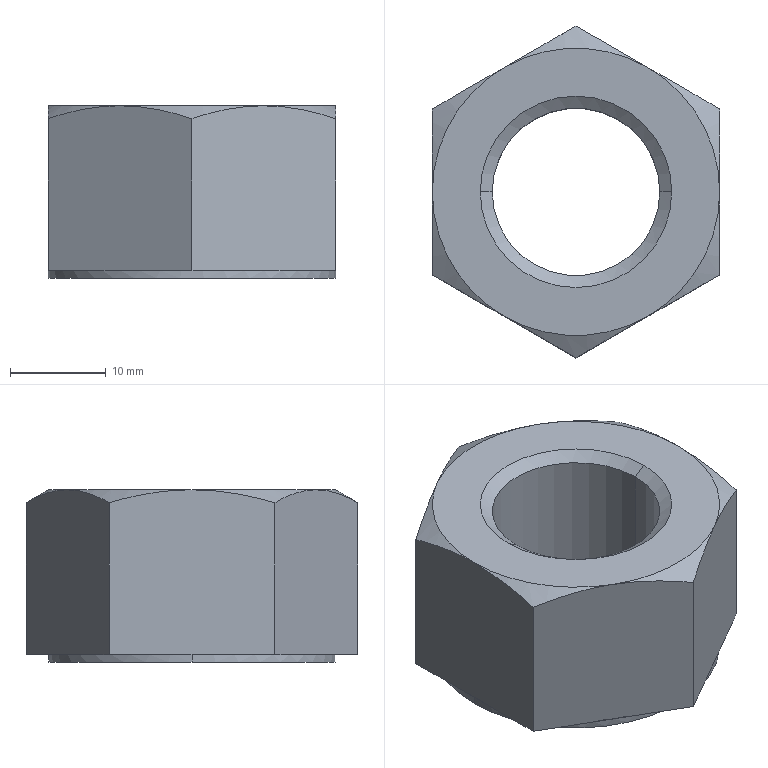Part | STEP file | hex nut style 1_am_B18.2.4.1M - Hex nut, Style 1,  M20 x 2.5 --W-N | 1 solid | 30 faces | box 30 x 34.641 x 18 mm | volume 9548 mm3 | plane 14 | cone 10 | cylinder 6 | commonest cylinder face diameters 17.5 x2 20 x2 30 x2